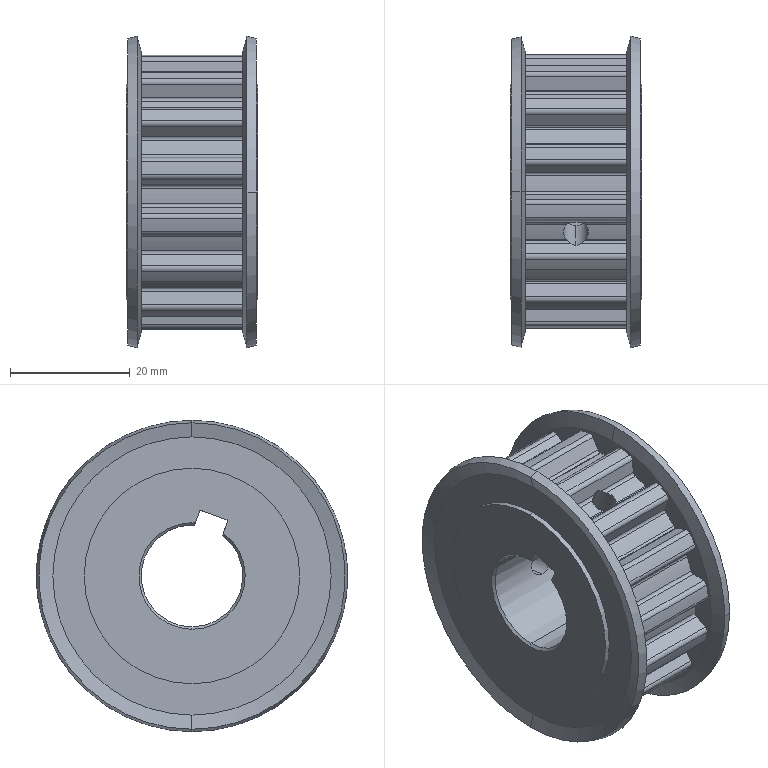Part | SolidWorks | features BaseBody 1 | 1 solid | 179 faces | box 22 x 52 x 52 mm | volume 27183 mm3 | cylinder 122 | plane 39 | cone 18 | commonest cylinder face diameters 1.2 x40 1.6 x37 39.5 x17 45.9 x15 4.134 x4 36 x4